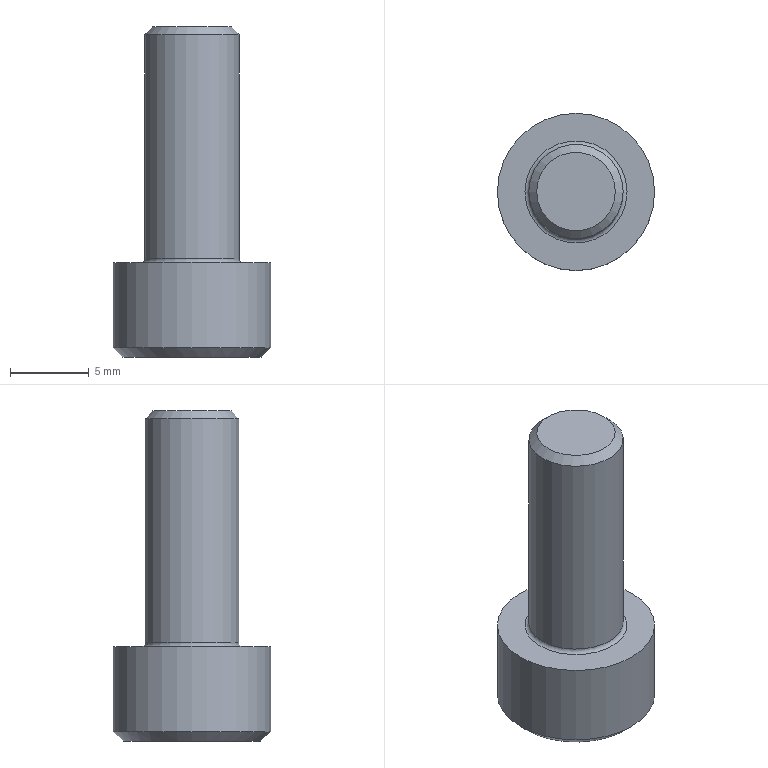Part | STEP file | solid 208 | 1 solid | 21 faces | box 10 x 10 x 21 mm | volume 822.719 mm3 | plane 10 | sphere 6 | cylinder 2 | cone 2 | torus 1 | commonest cylinder face diameters 6 x1 10 x1